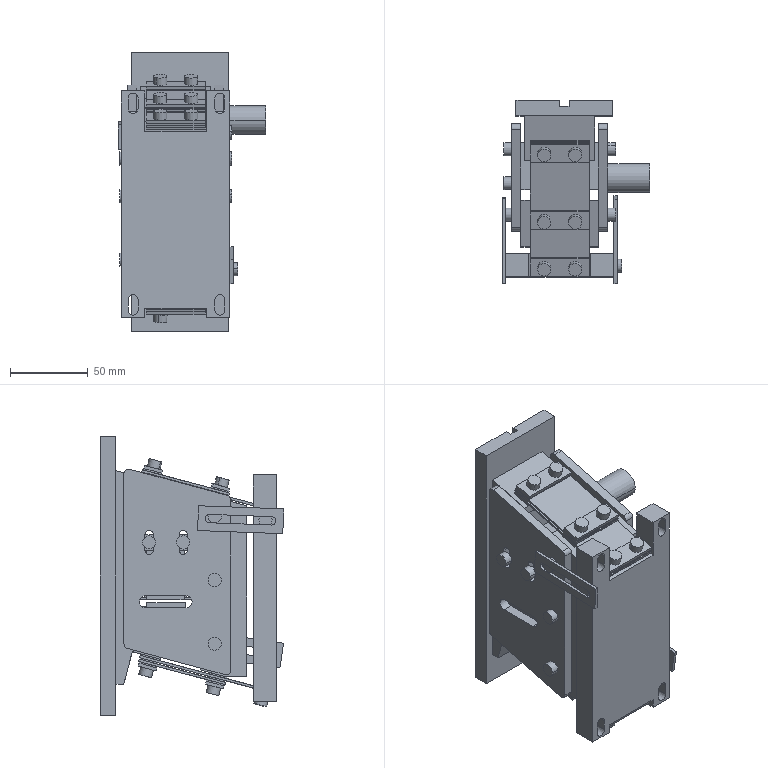Part | SolidWorks | features BaseBody 64 | 64 solids | 906 faces | box 95 x 118.301 x 180 mm | volume 694556 mm3 | plane 447 | cylinder 400 | cone 59 | commonest cylinder face diameters 6 x104 4.2 x68 5.4 x66 5 x52 8.5 x52 2 x30